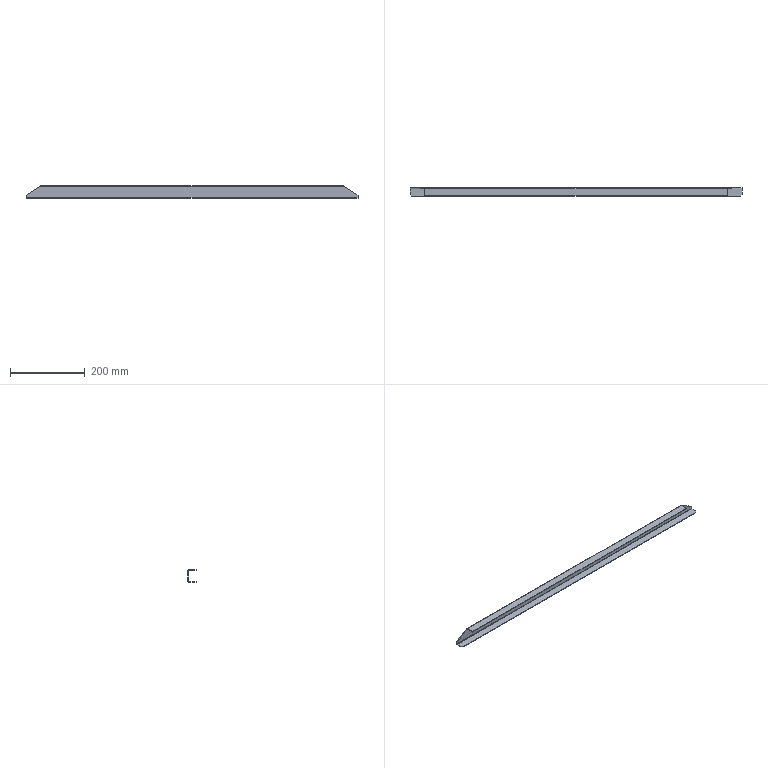Part | STEP file | b-015 | 1 solid | 33 faces | box 890 x 21.5 x 33 mm | volume 91888 mm3 | plane 20 | spline 9 | cylinder 4 | commonest cylinder face diameters 1.473 x2 4.473 x2